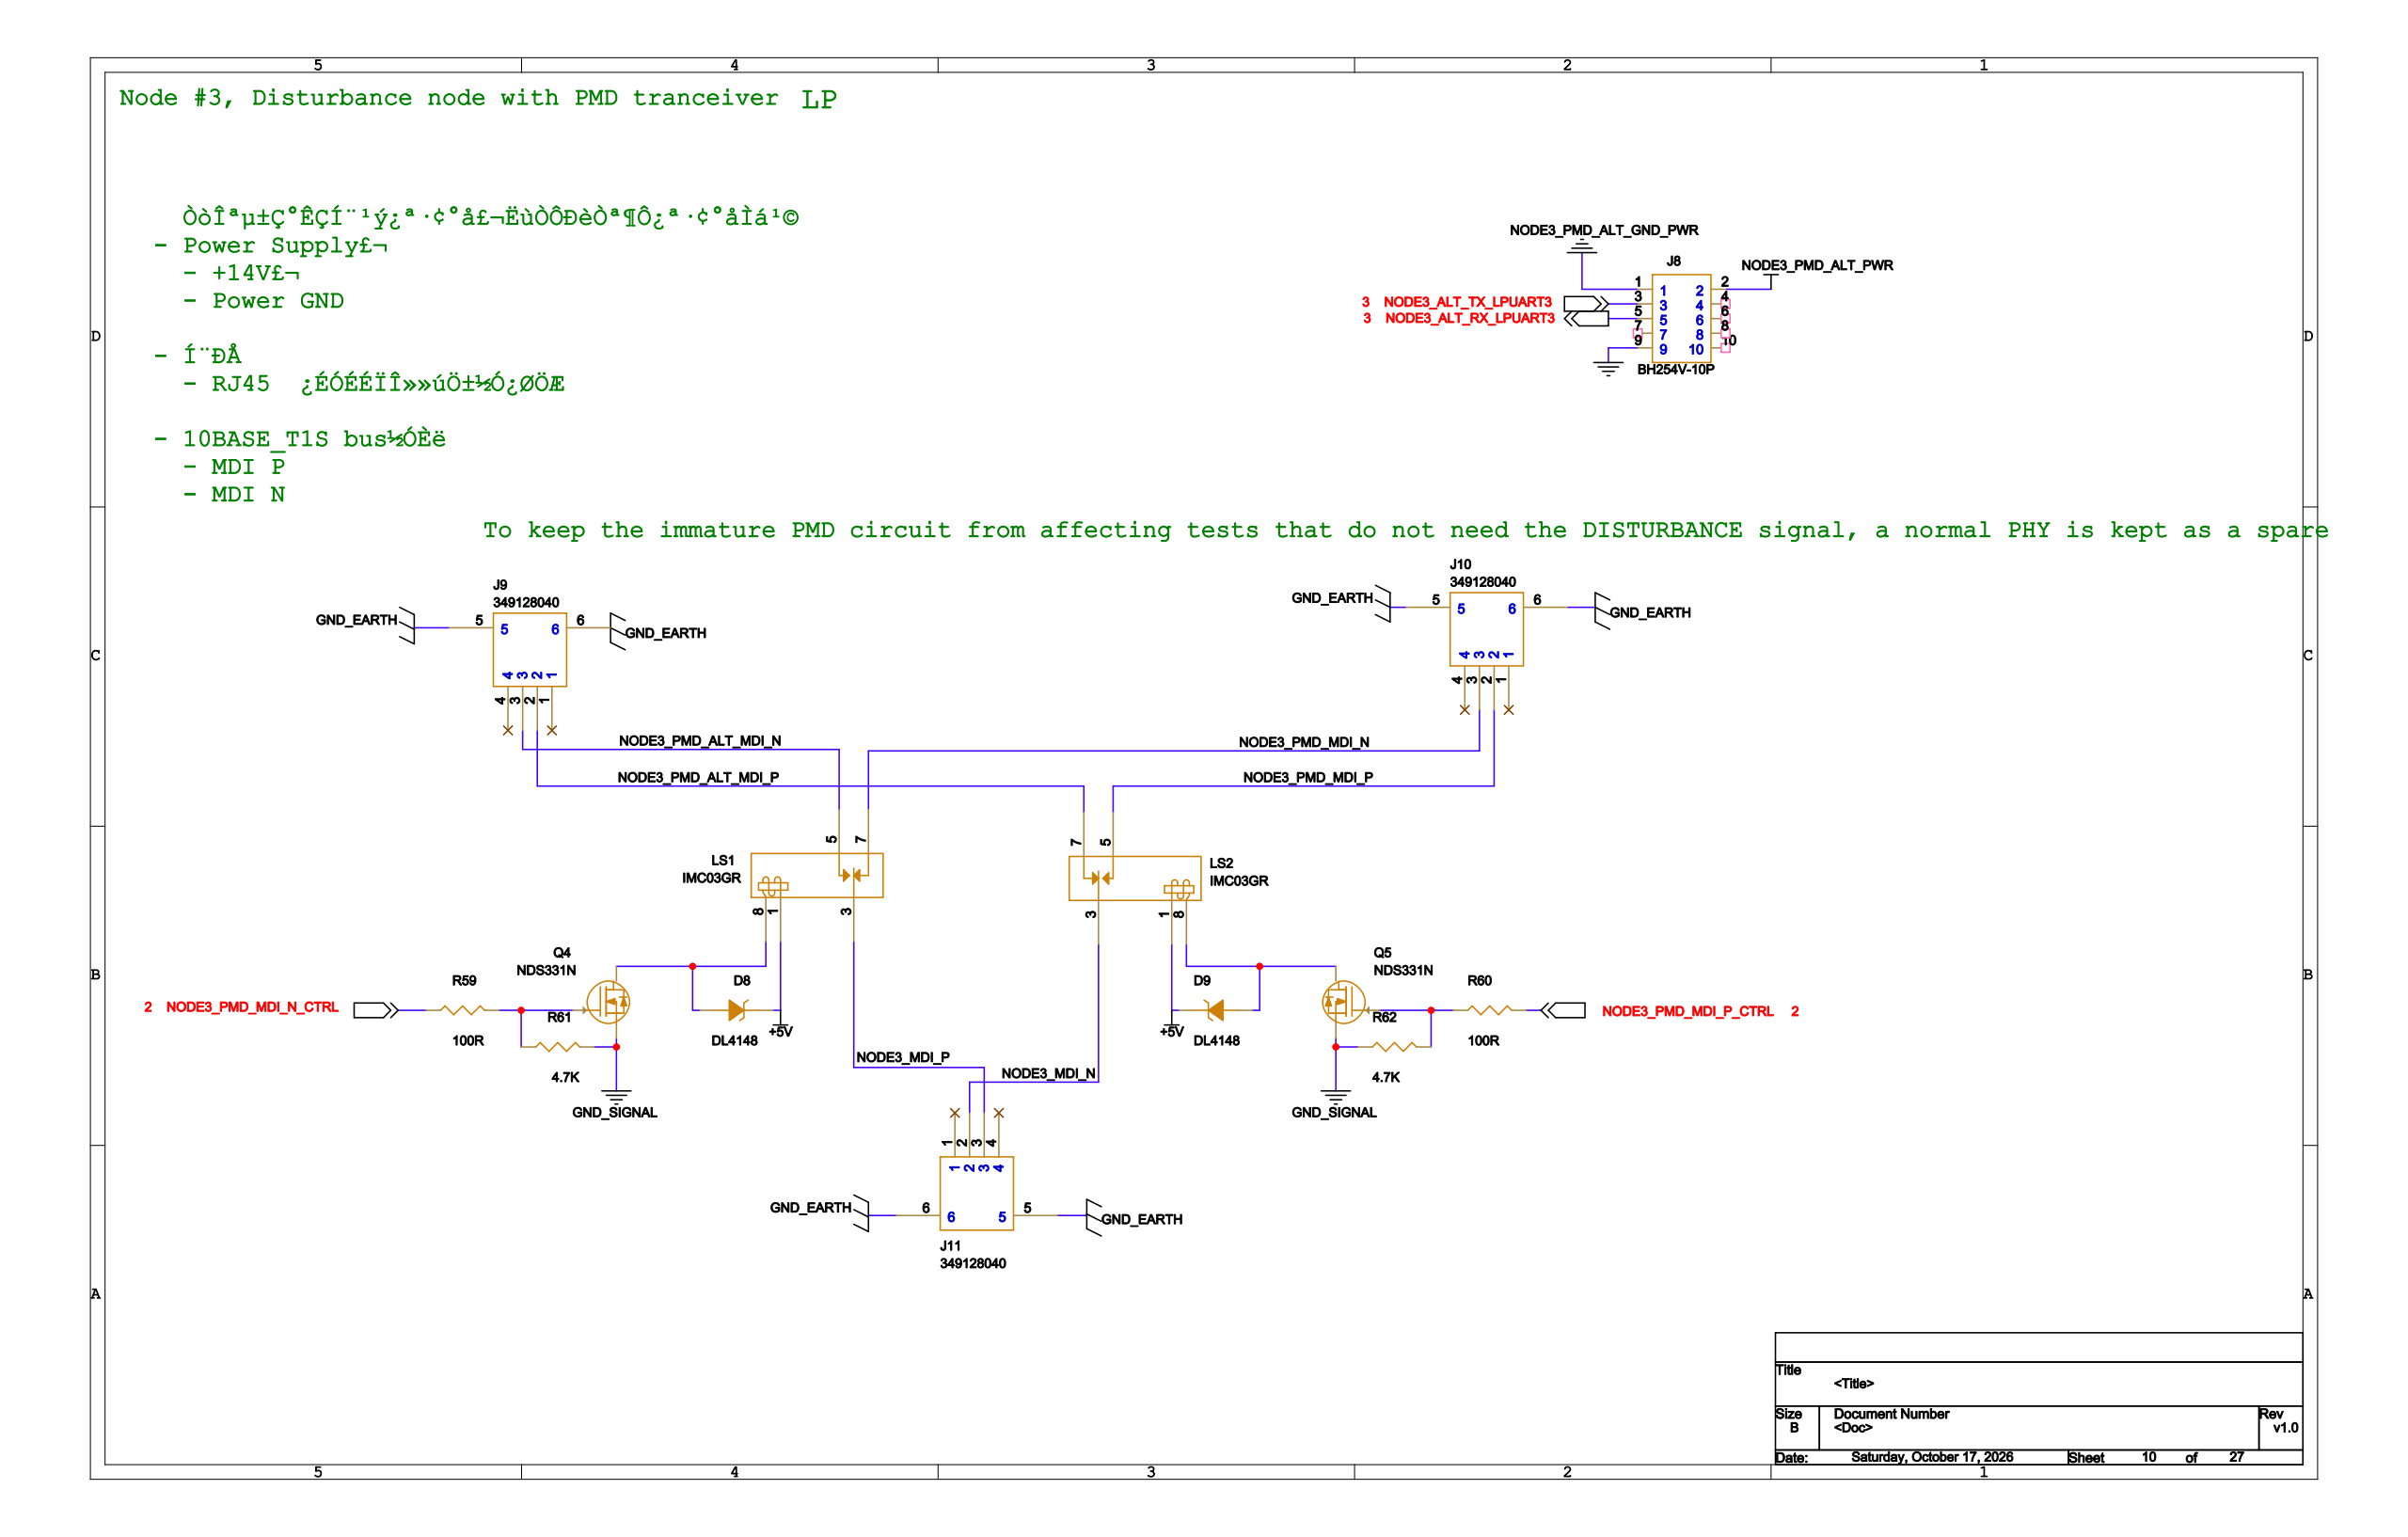Circuit board | Cadence Allegro | 477 parts | 327 nets | one sheet of the schematic
Parts on this sheet (reference | value | footprint):
D8 | DL4148 | MINIMELF
D9 | DL4148 | MINIMELF
J8 | BH254V-10P | BH254V-10P
J9 | 349128040 | 349128040
J10 | 349128040 | 349128040
J11 | 349128040 | 349128040
LS1 | IMC03GR | IMC03GR
LS2 | IMC03GR | IMC03GR
Q4 | NDS331N | SOT23-3
Q5 | NDS331N | SOT23-3
R59 | 100R | R0402
R60 | 100R | R0402
R61 | 4.7K | R0402
R62 | 4.7K | R0402
Nets of these parts (net: part-pin ...):
N16921593: Q4-1 R59-1 R61-2
NODE3_PMD_MDI_N_CTRL: R59-2
N16920900: Q5-1 R60-1 R62-2
NODE3_PMD_MDI_P_CTRL: R60-2
GND: J8-9
BAT_GND: Q4-2 Q5-2 R61-1 R62-1
GND_EARTH: J9-5 J9-6 J10-5 J10-6 J11-5 J11-6
+5V: D8-2 D9-2 LS1-1 LS2-1
N16921547: D8-1 LS1-8 Q4-3
N16920860: D9-1 LS2-8 Q5-3
NODE3_PMD_ALT_GND_PWR: J8-1
NODE3_PMD_ALT_PWR: J8-2
NODE3_ALT_TX_LPUART3: J8-3
NODE3_ALT_RX_LPUART3: J8-5
NODE3_PMD_MDI_P: J10-2 LS2-5
NODE3_PMD_MDI_N: J10-3 LS1-7
NODE3_MDI_N: J11-2 LS2-3
NODE3_MDI_P: J11-3 LS1-3
NODE3_PMD_ALT_MDI_P: J9-2 LS2-7
NODE3_PMD_ALT_MDI_N: J9-3 LS1-5